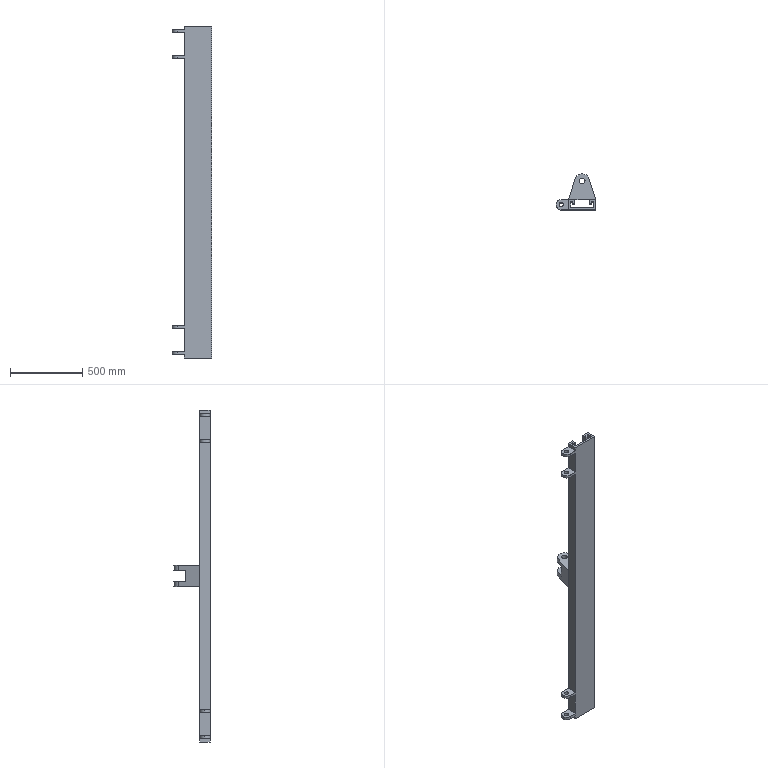Part | SolidWorks | 1 solid | 60 faces | box 275 x 250 x 2300 mm | volume 16623350 mm3 | plane 40 | cylinder 20 | commonest cylinder face diameters 30 x8 70 x6 40 x4 100 x2